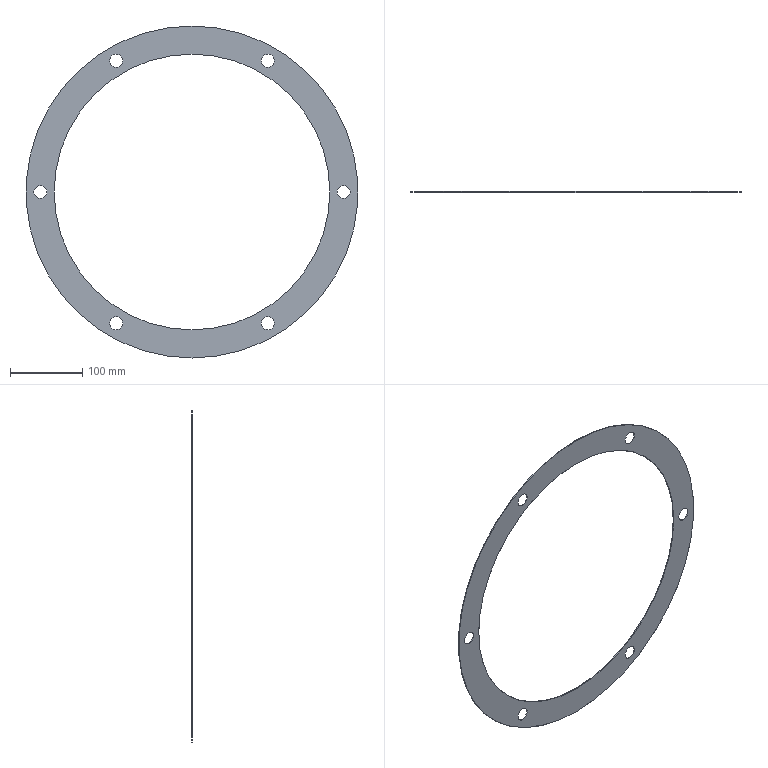Part | SolidWorks | features CirPattern 1, Extrusion 1, ICE 1 | 1 solid | 18 faces | box 460 x 1 x 460 mm | volume 50055 mm3 | cylinder 16 | plane 2 | commonest cylinder face diameters 18 x12 382 x2 460 x2
STEP:
#1=CARTESIAN_POINT('',(-105.,0.5,-190.865));
#2=VERTEX_POINT('',#1);
#3=CARTESIAN_POINT('',(-105.,0.5,-172.865));
#4=VERTEX_POINT('',#3);
#5=CARTESIAN_POINT('',(-105.,0.5,-181.865));
#6=DIRECTION('',(0.,1.,0.));
#7=DIRECTION('',(-0.866,0.,0.5));
#8=AXIS2_PLACEMENT_3D('',#5,#6,#7);
#9=CIRCLE('',#8,9.);
#10=EDGE_CURVE('',#2,#4,#9,.T.);
#11=ORIENTED_EDGE('',*,*,#10,.T.);
#12=CARTESIAN_POINT('',(-105.,-0.5,-172.865));
#13=VERTEX_POINT('',#12);
#14=CARTESIAN_POINT('',(-105.,0.5,-172.865));
#15=DIRECTION('',(0.,-1.,0.));
#16=VECTOR('',#15,1000.);
#17=LINE('',#14,#16);
#18=EDGE_CURVE('',#4,#13,#17,.T.);
#19=ORIENTED_EDGE('',*,*,#18,.T.);
#20=CARTESIAN_POINT('',(-105.,-0.5,-190.865));
#21=VERTEX_POINT('',#20);
#22=CARTESIAN_POINT('',(-105.,-0.5,-181.865));
#23=DIRECTION('',(0.,1.,0.));
#24=DIRECTION('',(-0.866,0.,0.5));
#25=AXIS2_PLACEMENT_3D('',#22,#23,#24);
#26=CIRCLE('',#25,9.);
#27=EDGE_CURVE('',#21,#13,#26,.T.);
#28=ORIENTED_EDGE('',*,*,#27,.F.);
#29=CARTESIAN_POINT('',(-105.,0.5,-190.865));
#30=DIRECTION('',(0.,-1.,0.));
#31=VECTOR('',#30,1000.);
#32=LINE('',#29,#31);
#33=EDGE_CURVE('',#2,#21,#32,.T.);
#34=ORIENTED_EDGE('',*,*,#33,.F.);
#35=EDGE_LOOP('',(#11,#19,#28,#34));
#36=FACE_OUTER_BOUND('',#35,.T.);
#37=CARTESIAN_POINT('',(-105.,0.5,-181.865));
#38=DIRECTION('',(0.,-1.,0.));
#39=DIRECTION('',(0.,0.,-1.));
#40=AXIS2_PLACEMENT_3D('',#37,#38,#39);
#41=CYLINDRICAL_SURFACE('',#40,9.);
#42=ADVANCED_FACE('',(#36),#41,.F.);
#43=CARTESIAN_POINT('',(105.,0.5,-190.865));
#44=VERTEX_POINT('',#43);
#45=CARTESIAN_POINT('',(105.,0.5,-172.865));
#46=VERTEX_POINT('',#45);
#47=CARTESIAN_POINT('',(105.,0.5,-181.865));
#48=DIRECTION('',(0.,1.,0.));
#49=DIRECTION('',(-0.866,0.,-0.5));
#50=AXIS2_PLACEMENT_3D('',#47,#48,#49);
#51=CIRCLE('',#50,9.);
#52=EDGE_CURVE('',#44,#46,#51,.T.);
#53=ORIENTED_EDGE('',*,*,#52,.T.);
#54=CARTESIAN_POINT('',(105.,-0.5,-172.865));
#55=VERTEX_POINT('',#54);
#56=CARTESIAN_POINT('',(105.,0.5,-172.865));
#57=DIRECTION('',(0.,-1.,0.));
#58=VECTOR('',#57,1000.);
#59=LINE('',#56,#58);
#60=EDGE_CURVE('',#46,#55,#59,.T.);
#61=ORIENTED_EDGE('',*,*,#60,.T.);
#62=CARTESIAN_POINT('',(105.,-0.5,-190.865));
#63=VERTEX_POINT('',#62);
#64=CARTESIAN_POINT('',(105.,-0.5,-181.865));
#65=DIRECTION('',(0.,1.,0.));
#66=DIRECTION('',(-0.866,0.,-0.5));
#67=AXIS2_PLACEMENT_3D('',#64,#65,#66);
#68=CIRCLE('',#67,9.);
#69=EDGE_CURVE('',#63,#55,#68,.T.);
#70=ORIENTED_EDGE('',*,*,#69,.F.);
#71=CARTESIAN_POINT('',(105.,0.5,-190.865));
#72=DIRECTION('',(0.,-1.,0.));
#73=VECTOR('',#72,1000.);
#74=LINE('',#71,#73);
#75=EDGE_CURVE('',#44,#63,#74,.T.);
#76=ORIENTED_EDGE('',*,*,#75,.F.);
#77=EDGE_LOOP('',(#53,#61,#70,#76));
#78=FACE_OUTER_BOUND('',#77,.T.);
#79=CARTESIAN_POINT('',(105.,0.5,-181.865));
#80=DIRECTION('',(0.,-1.,0.));
#81=DIRECTION('',(0.,0.,-1.));
#82=AXIS2_PLACEMENT_3D('',#79,#80,#81);
#83=CYLINDRICAL_SURFACE('',#82,9.);
#84=ADVANCED_FACE('',(#78),#83,.F.);
#85=CARTESIAN_POINT('',(210.,0.5,-9.));
#86=VERTEX_POINT('',#85);
#87=CARTESIAN_POINT('',(210.,0.5,9.));
#88=VERTEX_POINT('',#87);
#89=CARTESIAN_POINT('',(210.,0.5,0.));
#90=DIRECTION('',(0.,1.,0.));
#91=DIRECTION('',(0.,0.,-1.));
#92=AXIS2_PLACEMENT_3D('',#89,#90,#91);
#93=CIRCLE('',#92,9.);
#94=EDGE_CURVE('',#86,#88,#93,.T.);
#95=ORIENTED_EDGE('',*,*,#94,.T.);
#96=CARTESIAN_POINT('',(210.,-0.5,9.));
#97=VERTEX_POINT('',#96);
#98=CARTESIAN_POINT('',(210.,0.5,9.));
#99=DIRECTION('',(0.,-1.,0.));
#100=VECTOR('',#99,1000.);
#101=LINE('',#98,#100);
#102=EDGE_CURVE('',#88,#97,#101,.T.);
#103=ORIENTED_EDGE('',*,*,#102,.T.);
#104=CARTESIAN_POINT('',(210.,-0.5,-9.));
#105=VERTEX_POINT('',#104);
#106=CARTESIAN_POINT('',(210.,-0.5,0.));
#107=DIRECTION('',(0.,1.,0.));
#108=DIRECTION('',(0.,0.,-1.));
#109=AXIS2_PLACEMENT_3D('',#106,#107,#108);
#110=CIRCLE('',#109,9.);
#111=EDGE_CURVE('',#105,#97,#110,.T.);
#112=ORIENTED_EDGE('',*,*,#111,.F.);
#113=CARTESIAN_POINT('',(210.,0.5,-9.));
#114=DIRECTION('',(0.,-1.,0.));
#115=VECTOR('',#114,1000.);
#116=LINE('',#113,#115);
#117=EDGE_CURVE('',#86,#105,#116,.T.);
#118=ORIENTED_EDGE('',*,*,#117,.F.);
#119=EDGE_LOOP('',(#95,#103,#112,#118));
#120=FACE_OUTER_BOUND('',#119,.T.);
#121=CARTESIAN_POINT('',(210.,0.5,0.));
#122=DIRECTION('',(0.,-1.,0.));
#123=DIRECTION('',(0.,0.,-1.));
#124=AXIS2_PLACEMENT_3D('',#121,#122,#123);
#125=CYLINDRICAL_SURFACE('',#124,9.);
#126=ADVANCED_FACE('',(#120),#125,.F.);
#127=CARTESIAN_POINT('',(105.,0.5,172.865));
#128=VERTEX_POINT('',#127);
#129=CARTESIAN_POINT('',(105.,0.5,190.865));
#130=VERTEX_POINT('',#129);
#131=CARTESIAN_POINT('',(105.,0.5,181.865));
#132=DIRECTION('',(0.,1.,0.));
#133=DIRECTION('',(0.866,0.,-0.5));
#134=AXIS2_PLACEMENT_3D('',#131,#132,#133);
#135=CIRCLE('',#134,9.);
#136=EDGE_CURVE('',#128,#130,#135,.T.);
#137=ORIENTED_EDGE('',*,*,#136,.T.);
#138=CARTESIAN_POINT('',(105.,-0.5,190.865));
#139=VERTEX_POINT('',#138);
#140=CARTESIAN_POINT('',(105.,0.5,190.865));
#141=DIRECTION('',(0.,-1.,0.));
#142=VECTOR('',#141,1000.);
#143=LINE('',#140,#142);
#144=EDGE_CURVE('',#130,#139,#143,.T.);
#145=ORIENTED_EDGE('',*,*,#144,.T.);
#146=CARTESIAN_POINT('',(105.,-0.5,172.865));
#147=VERTEX_POINT('',#146);
#148=CARTESIAN_POINT('',(105.,-0.5,181.865));
#149=DIRECTION('',(0.,1.,0.));
#150=DIRECTION('',(0.866,0.,-0.5));
#151=AXIS2_PLACEMENT_3D('',#148,#149,#150);
#152=CIRCLE('',#151,9.);
#153=EDGE_CURVE('',#147,#139,#152,.T.);
#154=ORIENTED_EDGE('',*,*,#153,.F.);
#155=CARTESIAN_POINT('',(105.,0.5,172.865));
#156=DIRECTION('',(0.,-1.,0.));
#157=VECTOR('',#156,1000.);
#158=LINE('',#155,#157);
#159=EDGE_CURVE('',#128,#147,#158,.T.);
#160=ORIENTED_EDGE('',*,*,#159,.F.);
#161=EDGE_LOOP('',(#137,#145,#154,#160));
#162=FACE_OUTER_BOUND('',#161,.T.);
#163=CARTESIAN_POINT('',(105.,0.5,181.865));
#164=DIRECTION('',(0.,-1.,0.));
#165=DIRECTION('',(0.,0.,-1.));
#166=AXIS2_PLACEMENT_3D('',#163,#164,#165);
#167=CYLINDRICAL_SURFACE('',#166,9.);
#168=ADVANCED_FACE('',(#162),#167,.F.);
#169=CARTESIAN_POINT('',(-105.,0.5,172.865));
#170=VERTEX_POINT('',#169);
#171=CARTESIAN_POINT('',(-105.,0.5,190.865));
#172=VERTEX_POINT('',#171);
#173=CARTESIAN_POINT('',(-105.,0.5,181.865));
#174=DIRECTION('',(0.,1.,0.));
#175=DIRECTION('',(0.866,0.,0.5));
#176=AXIS2_PLACEMENT_3D('',#173,#174,#175);
#177=CIRCLE('',#176,9.);
#178=EDGE_CURVE('',#170,#172,#177,.T.);
#179=ORIENTED_EDGE('',*,*,#178,.T.);
#180=CARTESIAN_POINT('',(-105.,-0.5,190.865));
#181=VERTEX_POINT('',#180);
#182=CARTESIAN_POINT('',(-105.,0.5,190.865));
#183=DIRECTION('',(0.,-1.,0.));
#184=VECTOR('',#183,1000.);
#185=LINE('',#182,#184);
#186=EDGE_CURVE('',#172,#181,#185,.T.);
#187=ORIENTED_EDGE('',*,*,#186,.T.);
#188=CARTESIAN_POINT('',(-105.,-0.5,172.865));
#189=VERTEX_POINT('',#188);
#190=CARTESIAN_POINT('',(-105.,-0.5,181.865));
#191=DIRECTION('',(0.,1.,0.));
#192=DIRECTION('',(0.866,0.,0.5));
#193=AXIS2_PLACEMENT_3D('',#190,#191,#192);
#194=CIRCLE('',#193,9.);
#195=EDGE_CURVE('',#189,#181,#194,.T.);
#196=ORIENTED_EDGE('',*,*,#195,.F.);
#197=CARTESIAN_POINT('',(-105.,0.5,172.865));
#198=DIRECTION('',(0.,-1.,0.));
#199=VECTOR('',#198,1000.);
#200=LINE('',#197,#199);
#201=EDGE_CURVE('',#170,#189,#200,.T.);
#202=ORIENTED_EDGE('',*,*,#201,.F.);
#203=EDGE_LOOP('',(#179,#187,#196,#202));
#204=FACE_OUTER_BOUND('',#203,.T.);
#205=CARTESIAN_POINT('',(-105.,0.5,181.865));
#206=DIRECTION('',(0.,-1.,0.));
#207=DIRECTION('',(0.,0.,-1.));
#208=AXIS2_PLACEMENT_3D('',#205,#206,#207);
#209=CYLINDRICAL_SURFACE('',#208,9.);
#210=ADVANCED_FACE('',(#204),#209,.F.);
#211=CARTESIAN_POINT('',(-210.,0.5,-9.));
#212=VERTEX_POINT('',#211);
#213=CARTESIAN_POINT('',(-210.,0.5,9.));
#214=VERTEX_POINT('',#213);
#215=CARTESIAN_POINT('',(-210.,0.5,0.));
#216=DIRECTION('',(0.,1.,0.));
#217=DIRECTION('',(0.,0.,1.));
#218=AXIS2_PLACEMENT_3D('',#215,#216,#217);
#219=CIRCLE('',#218,9.);
#220=EDGE_CURVE('',#212,#214,#219,.T.);
#221=ORIENTED_EDGE('',*,*,#220,.T.);
#222=CARTESIAN_POINT('',(-210.,-0.5,9.));
#223=VERTEX_POINT('',#222);
#224=CARTESIAN_POINT('',(-210.,0.5,9.));
#225=DIRECTION('',(0.,-1.,0.));
#226=VECTOR('',#225,1000.);
#227=LINE('',#224,#226);
#228=EDGE_CURVE('',#214,#223,#227,.T.);
#229=ORIENTED_EDGE('',*,*,#228,.T.);
#230=CARTESIAN_POINT('',(-210.,-0.5,-9.));
#231=VERTEX_POINT('',#230);
#232=CARTESIAN_POINT('',(-210.,-0.5,0.));
#233=DIRECTION('',(0.,1.,0.));
#234=DIRECTION('',(0.,0.,1.));
#235=AXIS2_PLACEMENT_3D('',#232,#233,#234);
#236=CIRCLE('',#235,9.);
#237=EDGE_CURVE('',#231,#223,#236,.T.);
#238=ORIENTED_EDGE('',*,*,#237,.F.);
#239=CARTESIAN_POINT('',(-210.,0.5,-9.));
#240=DIRECTION('',(0.,-1.,0.));
#241=VECTOR('',#240,1000.);
#242=LINE('',#239,#241);
#243=EDGE_CURVE('',#212,#231,#242,.T.);
#244=ORIENTED_EDGE('',*,*,#243,.F.);
#245=EDGE_LOOP('',(#221,#229,#238,#244));
#246=FACE_OUTER_BOUND('',#245,.T.);
#247=CARTESIAN_POINT('',(-210.,0.5,0.));
#248=DIRECTION('',(0.,-1.,0.));
#249=DIRECTION('',(0.,0.,-1.));
#250=AXIS2_PLACEMENT_3D('',#247,#248,#249);
#251=CYLINDRICAL_SURFACE('',#250,9.);
#252=ADVANCED_FACE('',(#246),#251,.F.);
#253=CARTESIAN_POINT('',(0.,0.5,-191.));
#254=VERTEX_POINT('',#253);
#255=CARTESIAN_POINT('',(0.,0.5,191.));
#256=VERTEX_POINT('',#255);
#257=CARTESIAN_POINT('',(0.,0.5,0.));
#258=DIRECTION('',(0.,1.,0.));
#259=DIRECTION('',(0.,0.,1.));
#260=AXIS2_PLACEMENT_3D('',#257,#258,#259);
#261=CIRCLE('',#260,191.);
#262=EDGE_CURVE('',#254,#256,#261,.T.);
#263=ORIENTED_EDGE('',*,*,#262,.T.);
#264=CARTESIAN_POINT('',(0.,-0.5,191.));
#265=VERTEX_POINT('',#264);
#266=CARTESIAN_POINT('',(0.,0.5,191.));
#267=DIRECTION('',(0.,-1.,0.));
#268=VECTOR('',#267,1000.);
#269=LINE('',#266,#268);
#270=EDGE_CURVE('',#256,#265,#269,.T.);
#271=ORIENTED_EDGE('',*,*,#270,.T.);
#272=CARTESIAN_POINT('',(0.,-0.5,-191.));
#273=VERTEX_POINT('',#272);
#274=CARTESIAN_POINT('',(0.,-0.5,0.));
#275=DIRECTION('',(0.,1.,0.));
#276=DIRECTION('',(0.,0.,1.));
#277=AXIS2_PLACEMENT_3D('',#274,#275,#276);
#278=CIRCLE('',#277,191.);
#279=EDGE_CURVE('',#273,#265,#278,.T.);
#280=ORIENTED_EDGE('',*,*,#279,.F.);
#281=CARTESIAN_POINT('',(0.,0.5,-191.));
#282=DIRECTION('',(0.,-1.,0.));
#283=VECTOR('',#282,1000.);
#284=LINE('',#281,#283);
#285=EDGE_CURVE('',#254,#273,#284,.T.);
#286=ORIENTED_EDGE('',*,*,#285,.F.);
#287=EDGE_LOOP('',(#263,#271,#280,#286));
#288=FACE_OUTER_BOUND('',#287,.T.);
#289=CARTESIAN_POINT('',(0.,0.5,0.));
#290=DIRECTION('',(0.,-1.,0.));
#291=DIRECTION('',(0.,0.,-1.));
#292=AXIS2_PLACEMENT_3D('',#289,#290,#291);
#293=CYLINDRICAL_SURFACE('',#292,191.);
#294=ADVANCED_FACE('',(#288),#293,.F.);
#295=CARTESIAN_POINT('',(0.,0.5,230.));
#296=VERTEX_POINT('',#295);
#297=CARTESIAN_POINT('',(0.,0.5,-230.));
#298=VERTEX_POINT('',#297);
#299=CARTESIAN_POINT('',(0.,0.5,0.));
#300=DIRECTION('',(0.,1.,0.));
#301=DIRECTION('',(0.,0.,1.));
#302=AXIS2_PLACEMENT_3D('',#299,#300,#301);
#303=CIRCLE('',#302,230.);
#304=EDGE_CURVE('',#296,#298,#303,.T.);
#305=ORIENTED_EDGE('',*,*,#304,.F.);
#306=CARTESIAN_POINT('',(0.,-0.5,230.));
#307=VERTEX_POINT('',#306);
#308=CARTESIAN_POINT('',(0.,0.5,230.));
#309=DIRECTION('',(0.,-1.,0.));
#310=VECTOR('',#309,1000.);
#311=LINE('',#308,#310);
#312=EDGE_CURVE('',#296,#307,#311,.T.);
#313=ORIENTED_EDGE('',*,*,#312,.T.);
#314=CARTESIAN_POINT('',(0.,-0.5,-230.));
#315=VERTEX_POINT('',#314);
#316=CARTESIAN_POINT('',(0.,-0.5,0.));
#317=DIRECTION('',(0.,1.,0.));
#318=DIRECTION('',(0.,0.,1.));
#319=AXIS2_PLACEMENT_3D('',#316,#317,#318);
#320=CIRCLE('',#319,230.);
#321=EDGE_CURVE('',#307,#315,#320,.T.);
#322=ORIENTED_EDGE('',*,*,#321,.T.);
#323=CARTESIAN_POINT('',(0.,0.5,-230.));
#324=DIRECTION('',(0.,-1.,0.));
#325=VECTOR('',#324,1000.);
#326=LINE('',#323,#325);
#327=EDGE_CURVE('',#298,#315,#326,.T.);
#328=ORIENTED_EDGE('',*,*,#327,.F.);
#329=EDGE_LOOP('',(#305,#313,#322,#328));
#330=FACE_OUTER_BOUND('',#329,.T.);
#331=CARTESIAN_POINT('',(0.,0.5,0.));
#332=DIRECTION('',(0.,-1.,0.));
#333=DIRECTION('',(0.,0.,-1.));
#334=AXIS2_PLACEMENT_3D('',#331,#332,#333);
#335=CYLINDRICAL_SURFACE('',#334,230.);
#336=ADVANCED_FACE('',(#330),#335,.T.);
#337=ORIENTED_EDGE('',*,*,#52,.F.);
#338=CARTESIAN_POINT('',(105.,0.5,-181.865));
#339=DIRECTION('',(0.,1.,0.));
#340=DIRECTION('',(-0.866,0.,-0.5));
#341=AXIS2_PLACEMENT_3D('',#338,#339,#340);
#342=CIRCLE('',#341,9.);
#343=EDGE_CURVE('',#46,#44,#342,.T.);
#344=ORIENTED_EDGE('',*,*,#343,.F.);
#345=EDGE_LOOP('',(#337,#344));
#346=FACE_BOUND('',#345,.T.);
#347=ORIENTED_EDGE('',*,*,#136,.F.);
#348=CARTESIAN_POINT('',(105.,0.5,181.865));
#349=DIRECTION('',(0.,1.,0.));
#350=DIRECTION('',(0.866,0.,-0.5));
#351=AXIS2_PLACEMENT_3D('',#348,#349,#350);
#352=CIRCLE('',#351,9.);
#353=EDGE_CURVE('',#130,#128,#352,.T.);
#354=ORIENTED_EDGE('',*,*,#353,.F.);
#355=EDGE_LOOP('',(#347,#354));
#356=FACE_BOUND('',#355,.T.);
#357=ORIENTED_EDGE('',*,*,#220,.F.);
#358=CARTESIAN_POINT('',(-210.,0.5,0.));
#359=DIRECTION('',(0.,1.,0.));
#360=DIRECTION('',(0.,0.,1.));
#361=AXIS2_PLACEMENT_3D('',#358,#359,#360);
#362=CIRCLE('',#361,9.);
#363=EDGE_CURVE('',#214,#212,#362,.T.);
#364=ORIENTED_EDGE('',*,*,#363,.F.);
#365=EDGE_LOOP('',(#357,#364));
#366=FACE_BOUND('',#365,.T.);
#367=CARTESIAN_POINT('',(0.,0.5,0.));
#368=DIRECTION('',(0.,1.,0.));
#369=DIRECTION('',(0.,0.,1.));
#370=AXIS2_PLACEMENT_3D('',#367,#368,#369);
#371=CIRCLE('',#370,230.);
#372=EDGE_CURVE('',#298,#296,#371,.T.);
#373=ORIENTED_EDGE('',*,*,#372,.T.);
#374=ORIENTED_EDGE('',*,*,#304,.T.);
#375=EDGE_LOOP('',(#373,#374));
#376=FACE_OUTER_BOUND('',#375,.T.);
#377=ORIENTED_EDGE('',*,*,#262,.F.);
#378=CARTESIAN_POINT('',(0.,0.5,0.));
#379=DIRECTION('',(0.,1.,0.));
#380=DIRECTION('',(0.,0.,1.));
#381=AXIS2_PLACEMENT_3D('',#378,#379,#380);
#382=CIRCLE('',#381,191.);
#383=EDGE_CURVE('',#256,#254,#382,.T.);
#384=ORIENTED_EDGE('',*,*,#383,.F.);
#385=EDGE_LOOP('',(#377,#384));
#386=FACE_BOUND('',#385,.T.);
#387=ORIENTED_EDGE('',*,*,#178,.F.);
#388=CARTESIAN_POINT('',(-105.,0.5,181.865));
#389=DIRECTION('',(0.,1.,0.));
#390=DIRECTION('',(0.866,0.,0.5));
#391=AXIS2_PLACEMENT_3D('',#388,#389,#390);
#392=CIRCLE('',#391,9.);
#393=EDGE_CURVE('',#172,#170,#392,.T.);
#394=ORIENTED_EDGE('',*,*,#393,.F.);
#395=EDGE_LOOP('',(#387,#394));
#396=FACE_BOUND('',#395,.T.);
#397=ORIENTED_EDGE('',*,*,#94,.F.);
#398=CARTESIAN_POINT('',(210.,0.5,0.));
#399=DIRECTION('',(0.,1.,0.));
#400=DIRECTION('',(0.,0.,-1.));
#401=AXIS2_PLACEMENT_3D('',#398,#399,#400);
#402=CIRCLE('',#401,9.);
#403=EDGE_CURVE('',#88,#86,#402,.T.);
#404=ORIENTED_EDGE('',*,*,#403,.F.);
#405=EDGE_LOOP('',(#397,#404));
#406=FACE_BOUND('',#405,.T.);
#407=ORIENTED_EDGE('',*,*,#10,.F.);
#408=CARTESIAN_POINT('',(-105.,0.5,-181.865));
#409=DIRECTION('',(0.,1.,0.));
#410=DIRECTION('',(-0.866,0.,0.5));
#411=AXIS2_PLACEMENT_3D('',#408,#409,#410);
#412=CIRCLE('',#411,9.);
#413=EDGE_CURVE('',#4,#2,#412,.T.);
#414=ORIENTED_EDGE('',*,*,#413,.F.);
#415=EDGE_LOOP('',(#407,#414));
#416=FACE_BOUND('',#415,.T.);
#417=CARTESIAN_POINT('',(0.,0.5,0.));
#418=DIRECTION('',(0.,1.,0.));
#419=DIRECTION('',(0.,0.,1.));
#420=AXIS2_PLACEMENT_3D('',#417,#418,#419);
#421=PLANE('',#420);
#422=ADVANCED_FACE('',(#346,#356,#366,#376,#386,#396,#406,#416),#421,.T.);
#423=ORIENTED_EDGE('',*,*,#69,.T.);
#424=CARTESIAN_POINT('',(105.,-0.5,-181.865));
#425=DIRECTION('',(0.,1.,0.));
#426=DIRECTION('',(-0.866,0.,-0.5));
#427=AXIS2_PLACEMENT_3D('',#424,#425,#426);
#428=CIRCLE('',#427,9.);
#429=EDGE_CURVE('',#55,#63,#428,.T.);
#430=ORIENTED_EDGE('',*,*,#429,.T.);
#431=EDGE_LOOP('',(#423,#430));
#432=FACE_BOUND('',#431,.T.);
#433=ORIENTED_EDGE('',*,*,#153,.T.);
#434=CARTESIAN_POINT('',(105.,-0.5,181.865));
#435=DIRECTION('',(0.,1.,0.));
#436=DIRECTION('',(0.866,0.,-0.5));
#437=AXIS2_PLACEMENT_3D('',#434,#435,#436);
#438=CIRCLE('',#437,9.);
#439=EDGE_CURVE('',#139,#147,#438,.T.);
#440=ORIENTED_EDGE('',*,*,#439,.T.);
#441=EDGE_LOOP('',(#433,#440));
#442=FACE_BOUND('',#441,.T.);
#443=ORIENTED_EDGE('',*,*,#237,.T.);
#444=CARTESIAN_POINT('',(-210.,-0.5,0.));
#445=DIRECTION('',(0.,1.,0.));
#446=DIRECTION('',(0.,0.,1.));
#447=AXIS2_PLACEMENT_3D('',#444,#445,#446);
#448=CIRCLE('',#447,9.);
#449=EDGE_CURVE('',#223,#231,#448,.T.);
#450=ORIENTED_EDGE('',*,*,#449,.T.);
#451=EDGE_LOOP('',(#443,#450));
#452=FACE_BOUND('',#451,.T.);
#453=CARTESIAN_POINT('',(0.,-0.5,0.));
#454=DIRECTION('',(0.,1.,0.));
#455=DIRECTION('',(0.,0.,1.));
#456=AXIS2_PLACEMENT_3D('',#453,#454,#455);
#457=CIRCLE('',#456,230.);
#458=EDGE_CURVE('',#315,#307,#457,.T.);
#459=ORIENTED_EDGE('',*,*,#458,.F.);
#460=ORIENTED_EDGE('',*,*,#321,.F.);
#461=EDGE_LOOP('',(#459,#460));
#462=FACE_OUTER_BOUND('',#461,.T.);
#463=ORIENTED_EDGE('',*,*,#279,.T.);
#464=CARTESIAN_POINT('',(0.,-0.5,0.));
#465=DIRECTION('',(0.,1.,0.));
#466=DIRECTION('',(0.,0.,1.));
#467=AXIS2_PLACEMENT_3D('',#464,#465,#466);
#468=CIRCLE('',#467,191.);
#469=EDGE_CURVE('',#265,#273,#468,.T.);
#470=ORIENTED_EDGE('',*,*,#469,.T.);
#471=EDGE_LOOP('',(#463,#470));
#472=FACE_BOUND('',#471,.T.);
#473=ORIENTED_EDGE('',*,*,#195,.T.);
#474=CARTESIAN_POINT('',(-105.,-0.5,181.865));
#475=DIRECTION('',(0.,1.,0.));
#476=DIRECTION('',(0.866,0.,0.5));
#477=AXIS2_PLACEMENT_3D('',#474,#475,#476);
#478=CIRCLE('',#477,9.);
#479=EDGE_CURVE('',#181,#189,#478,.T.);
#480=ORIENTED_EDGE('',*,*,#479,.T.);
#481=EDGE_LOOP('',(#473,#480));
#482=FACE_BOUND('',#481,.T.);
#483=ORIENTED_EDGE('',*,*,#111,.T.);
#484=CARTESIAN_POINT('',(210.,-0.5,0.));
#485=DIRECTION('',(0.,1.,0.));
#486=DIRECTION('',(0.,0.,-1.));
#487=AXIS2_PLACEMENT_3D('',#484,#485,#486);
#488=CIRCLE('',#487,9.);
#489=EDGE_CURVE('',#97,#105,#488,.T.);
#490=ORIENTED_EDGE('',*,*,#489,.T.);
#491=EDGE_LOOP('',(#483,#490));
#492=FACE_BOUND('',#491,.T.);
#493=ORIENTED_EDGE('',*,*,#27,.T.);
#494=CARTESIAN_POINT('',(-105.,-0.5,-181.865));
#495=DIRECTION('',(0.,1.,0.));
#496=DIRECTION('',(-0.866,0.,0.5));
#497=AXIS2_PLACEMENT_3D('',#494,#495,#496);
#498=CIRCLE('',#497,9.);
#499=EDGE_CURVE('',#13,#21,#498,.T.);
#500=ORIENTED_EDGE('',*,*,#499,.T.);
#501=EDGE_LOOP('',(#493,#500));
#502=FACE_BOUND('',#501,.T.);
#503=CARTESIAN_POINT('',(0.,-0.5,0.));
#504=DIRECTION('',(0.,1.,0.));
#505=DIRECTION('',(0.,0.,1.));
#506=AXIS2_PLACEMENT_3D('',#503,#504,#505);
#507=PLANE('',#506);
#508=ADVANCED_FACE('',(#432,#442,#452,#462,#472,#482,#492,#502),#507,.F.);
#509=ORIENTED_EDGE('',*,*,#312,.F.);
#510=ORIENTED_EDGE('',*,*,#372,.F.);
#511=ORIENTED_EDGE('',*,*,#327,.T.);
#512=ORIENTED_EDGE('',*,*,#458,.T.);
#513=EDGE_LOOP('',(#509,#510,#511,#512));
#514=FACE_OUTER_BOUND('',#513,.T.);
#515=CARTESIAN_POINT('',(0.,0.5,0.));
#516=DIRECTION('',(0.,-1.,0.));
#517=DIRECTION('',(0.,0.,-1.));
#518=AXIS2_PLACEMENT_3D('',#515,#516,#517);
#519=CYLINDRICAL_SURFACE('',#518,230.);
#520=ADVANCED_FACE('',(#514),#519,.T.);
#521=ORIENTED_EDGE('',*,*,#270,.F.);
#522=ORIENTED_EDGE('',*,*,#383,.T.);
#523=ORIENTED_EDGE('',*,*,#285,.T.);
#524=ORIENTED_EDGE('',*,*,#469,.F.);
#525=EDGE_LOOP('',(#521,#522,#523,#524));
#526=FACE_OUTER_BOUND('',#525,.T.);
#527=CARTESIAN_POINT('',(0.,0.5,0.));
#528=DIRECTION('',(0.,-1.,0.));
#529=DIRECTION('',(0.,0.,-1.));
#530=AXIS2_PLACEMENT_3D('',#527,#528,#529);
#531=CYLINDRICAL_SURFACE('',#530,191.);
#532=ADVANCED_FACE('',(#526),#531,.F.);
#533=ORIENTED_EDGE('',*,*,#228,.F.);
#534=ORIENTED_EDGE('',*,*,#363,.T.);
#535=ORIENTED_EDGE('',*,*,#243,.T.);
#536=ORIENTED_EDGE('',*,*,#449,.F.);
#537=EDGE_LOOP('',(#533,#534,#535,#536));
#538=FACE_OUTER_BOUND('',#537,.T.);
#539=CARTESIAN_POINT('',(-210.,0.5,0.));
#540=DIRECTION('',(0.,-1.,0.));
#541=DIRECTION('',(0.,0.,-1.));
#542=AXIS2_PLACEMENT_3D('',#539,#540,#541);
#543=CYLINDRICAL_SURFACE('',#542,9.);
#544=ADVANCED_FACE('',(#538),#543,.F.);
#545=ORIENTED_EDGE('',*,*,#186,.F.);
#546=ORIENTED_EDGE('',*,*,#393,.T.);
#547=ORIENTED_EDGE('',*,*,#201,.T.);
#548=ORIENTED_EDGE('',*,*,#479,.F.);
#549=EDGE_LOOP('',(#545,#546,#547,#548));
#550=FACE_OUTER_BOUND('',#549,.T.);
#551=CARTESIAN_POINT('',(-105.,0.5,181.865));
#552=DIRECTION('',(0.,-1.,0.));
#553=DIRECTION('',(0.,0.,-1.));
#554=AXIS2_PLACEMENT_3D('',#551,#552,#553);
#555=CYLINDRICAL_SURFACE('',#554,9.);
#556=ADVANCED_FACE('',(#550),#555,.F.);
#557=ORIENTED_EDGE('',*,*,#144,.F.);
#558=ORIENTED_EDGE('',*,*,#353,.T.);
#559=ORIENTED_EDGE('',*,*,#159,.T.);
#560=ORIENTED_EDGE('',*,*,#439,.F.);
#561=EDGE_LOOP('',(#557,#558,#559,#560));
#562=FACE_OUTER_BOUND('',#561,.T.);
#563=CARTESIAN_POINT('',(105.,0.5,181.865));
#564=DIRECTION('',(0.,-1.,0.));
#565=DIRECTION('',(0.,0.,-1.));
#566=AXIS2_PLACEMENT_3D('',#563,#564,#565);
#567=CYLINDRICAL_SURFACE('',#566,9.);
#568=ADVANCED_FACE('',(#562),#567,.F.);
#569=ORIENTED_EDGE('',*,*,#102,.F.);
#570=ORIENTED_EDGE('',*,*,#403,.T.);
#571=ORIENTED_EDGE('',*,*,#117,.T.);
#572=ORIENTED_EDGE('',*,*,#489,.F.);
#573=EDGE_LOOP('',(#569,#570,#571,#572));
#574=FACE_OUTER_BOUND('',#573,.T.);
#575=CARTESIAN_POINT('',(210.,0.5,0.));
#576=DIRECTION('',(0.,-1.,0.));
#577=DIRECTION('',(0.,0.,-1.));
#578=AXIS2_PLACEMENT_3D('',#575,#576,#577);
#579=CYLINDRICAL_SURFACE('',#578,9.);
#580=ADVANCED_FACE('',(#574),#579,.F.);
#581=ORIENTED_EDGE('',*,*,#60,.F.);
#582=ORIENTED_EDGE('',*,*,#343,.T.);
#583=ORIENTED_EDGE('',*,*,#75,.T.);
#584=ORIENTED_EDGE('',*,*,#429,.F.);
#585=EDGE_LOOP('',(#581,#582,#583,#584));
#586=FACE_OUTER_BOUND('',#585,.T.);
#587=CARTESIAN_POINT('',(105.,0.5,-181.865));
#588=DIRECTION('',(0.,-1.,0.));
#589=DIRECTION('',(0.,0.,-1.));
#590=AXIS2_PLACEMENT_3D('',#587,#588,#589);
#591=CYLINDRICAL_SURFACE('',#590,9.);
#592=ADVANCED_FACE('',(#586),#591,.F.);
#593=ORIENTED_EDGE('',*,*,#18,.F.);
#594=ORIENTED_EDGE('',*,*,#413,.T.);
#595=ORIENTED_EDGE('',*,*,#33,.T.);
#596=ORIENTED_EDGE('',*,*,#499,.F.);
#597=EDGE_LOOP('',(#593,#594,#595,#596));
#598=FACE_OUTER_BOUND('',#597,.T.);
#599=CARTESIAN_POINT('',(-105.,0.5,-181.865));
#600=DIRECTION('',(0.,-1.,0.));
#601=DIRECTION('',(0.,0.,-1.));
#602=AXIS2_PLACEMENT_3D('',#599,#600,#601);
#603=CYLINDRICAL_SURFACE('',#602,9.);
#604=ADVANCED_FACE('',(#598),#603,.F.);
#605=CLOSED_SHELL('',(#42,#84,#126,#168,#210,#252,#294,#336,#422,#508,#520,#532,#544,#556,#568,#580,#592,#604));
#606=MANIFOLD_SOLID_BREP('',#605);
#607=CARTESIAN_POINT('',(0.,0.,0.));
#608=DIRECTION('',(0.,0.,1.));
#609=DIRECTION('',(1.,0.,0.));
#610=AXIS2_PLACEMENT_3D('',#607,#608,#609);
#611=(LENGTH_UNIT()NAMED_UNIT(*)SI_UNIT(.MILLI.,.METRE.));
#612=UNCERTAINTY_MEASURE_WITH_UNIT(LENGTH_MEASURE(0.00001),#611,'','');
#613=(NAMED_UNIT(*)PLANE_ANGLE_UNIT()SI_UNIT($,.RADIAN.));
#614=(NAMED_UNIT(*)SI_UNIT($,.STERADIAN.)SOLID_ANGLE_UNIT());
#615=(GEOMETRIC_REPRESENTATION_CONTEXT(3)GLOBAL_UNCERTAINTY_ASSIGNED_CONTEXT((#612))GLOBAL_UNIT_ASSIGNED_CONTEXT((#611,#613,#614))REPRESENTATION_CONTEXT('',''));
#616=ADVANCED_BREP_SHAPE_REPRESENTATION('',(#606,#610),#615);